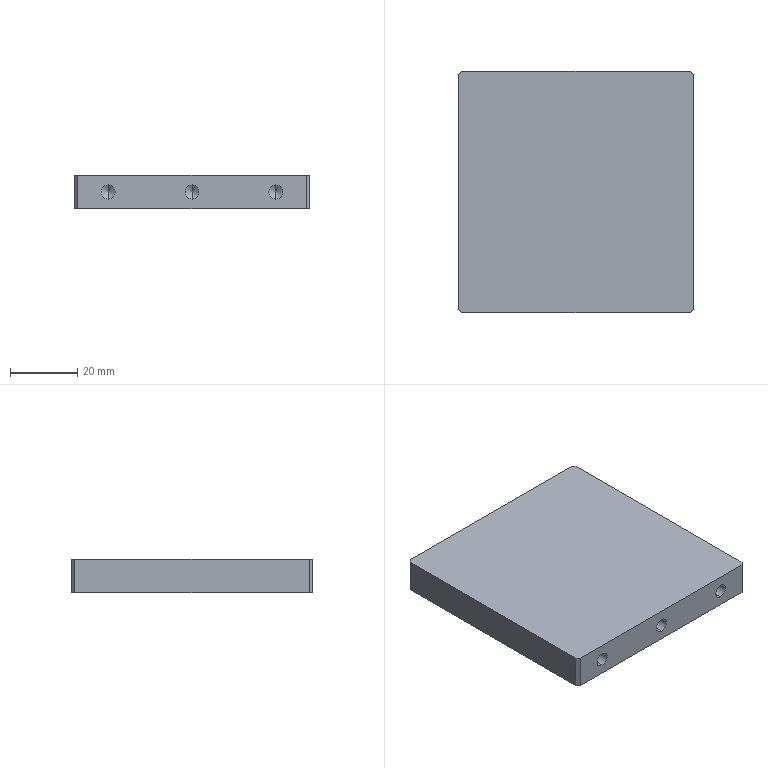Part | STEP file | support plate 70 | 1 solid | 34 faces | box 70 x 72 x 10 mm | volume 49181 mm3 | cylinder 12 | cone 12 | plane 10 | commonest cylinder face diameters 4.2 x12